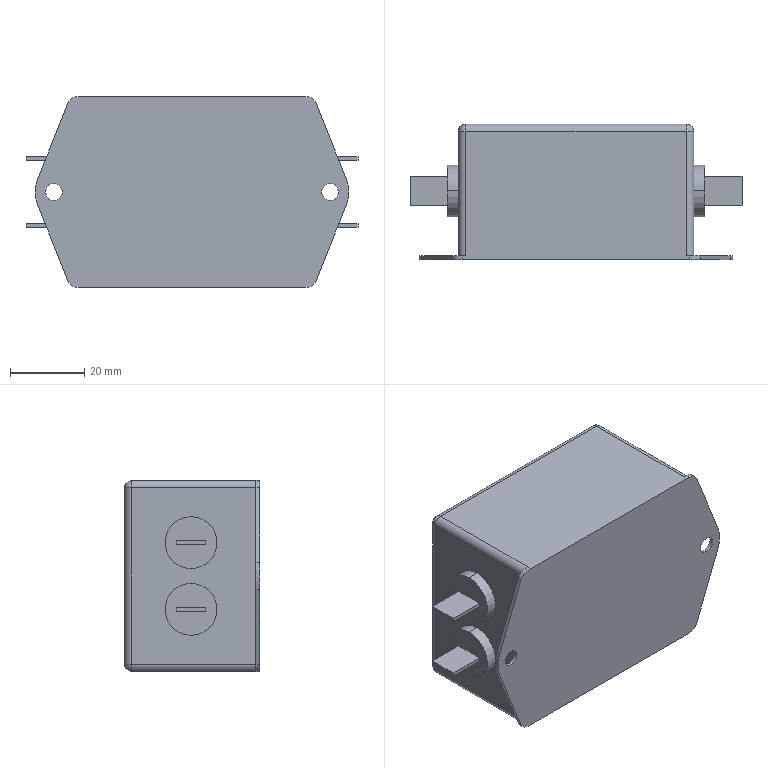Part | STEP file | Power filter DL-10T1 | 1 solid | 127 faces | box 89.5 x 36.5 x 51.5 mm | volume 121807 mm3 | plane 81 | cylinder 26 | spline 16 | sphere 4 | commonest cylinder face diameters 4 x8 14 x8 4.5 x4 6 x4 20 x2